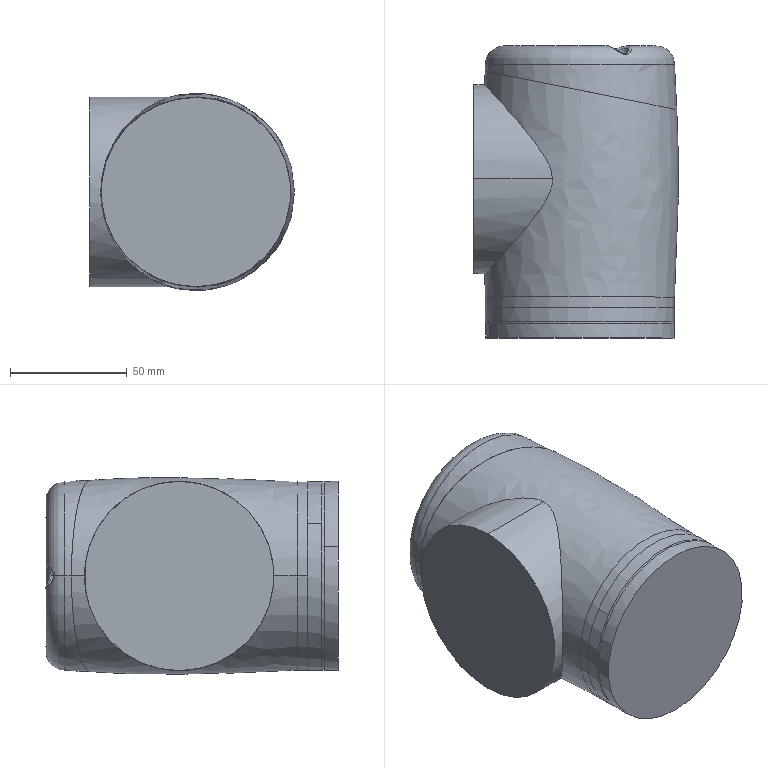Part | SolidWorks | features BaseBody 2, Fillet 1, ICE 1 | 2 solids | 89 faces | box 87.688 x 125 x 84.375 mm | volume 705522 mm3 | plane 50 | spline 18 | cylinder 17 | torus 4 | commonest cylinder face diameters 81 x10 8 x7